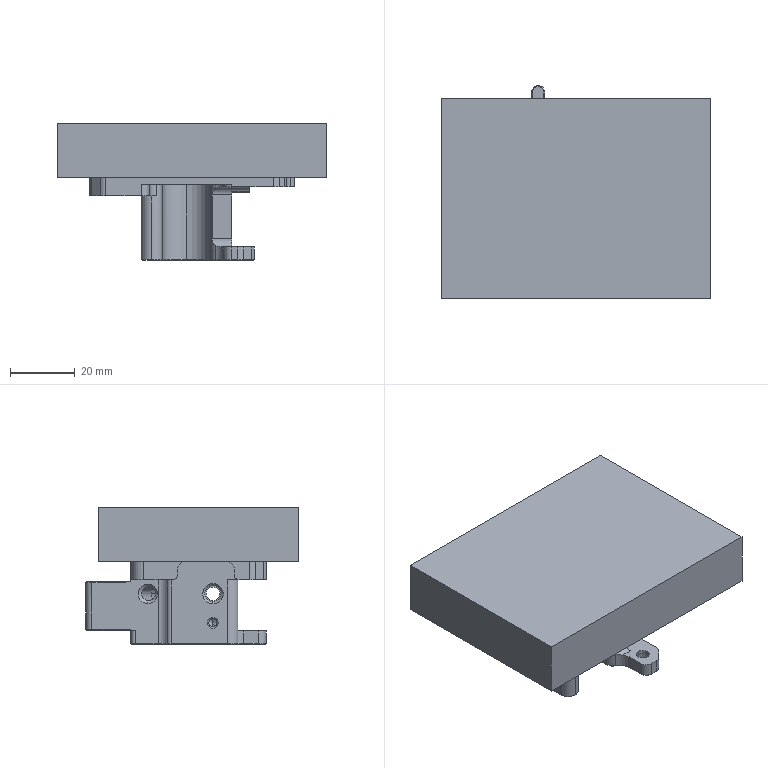Part | 3 solids | 790 faces | box 83.5 x 66 x 42.45 mm | volume 124721 mm3 | cylinder 276 | plane 274 | cone 236 | spline 4 | commonest cylinder face diameters 5 x54 4 x36 6 x34 2.5 x28 6.5 x22 3 x14